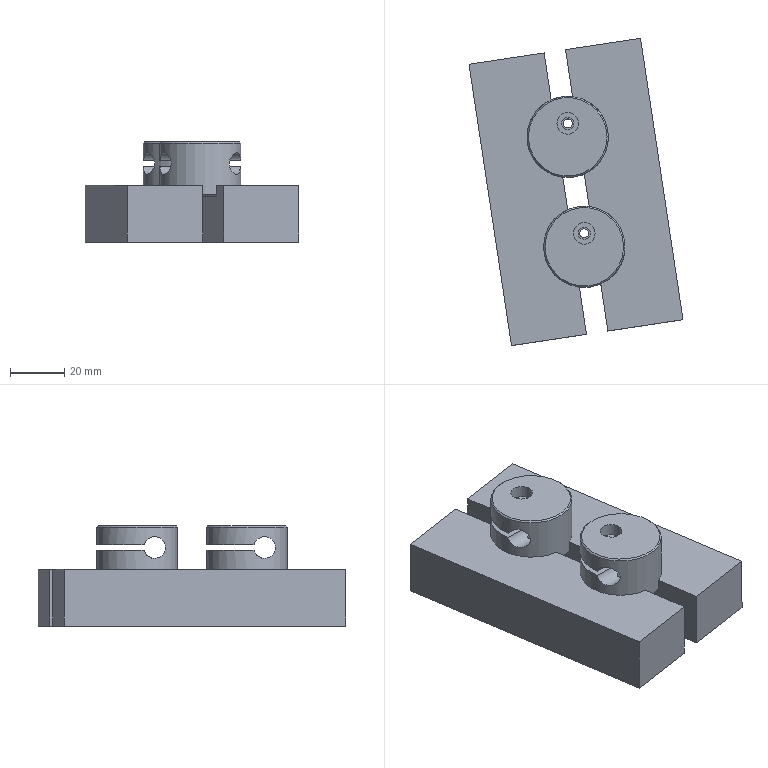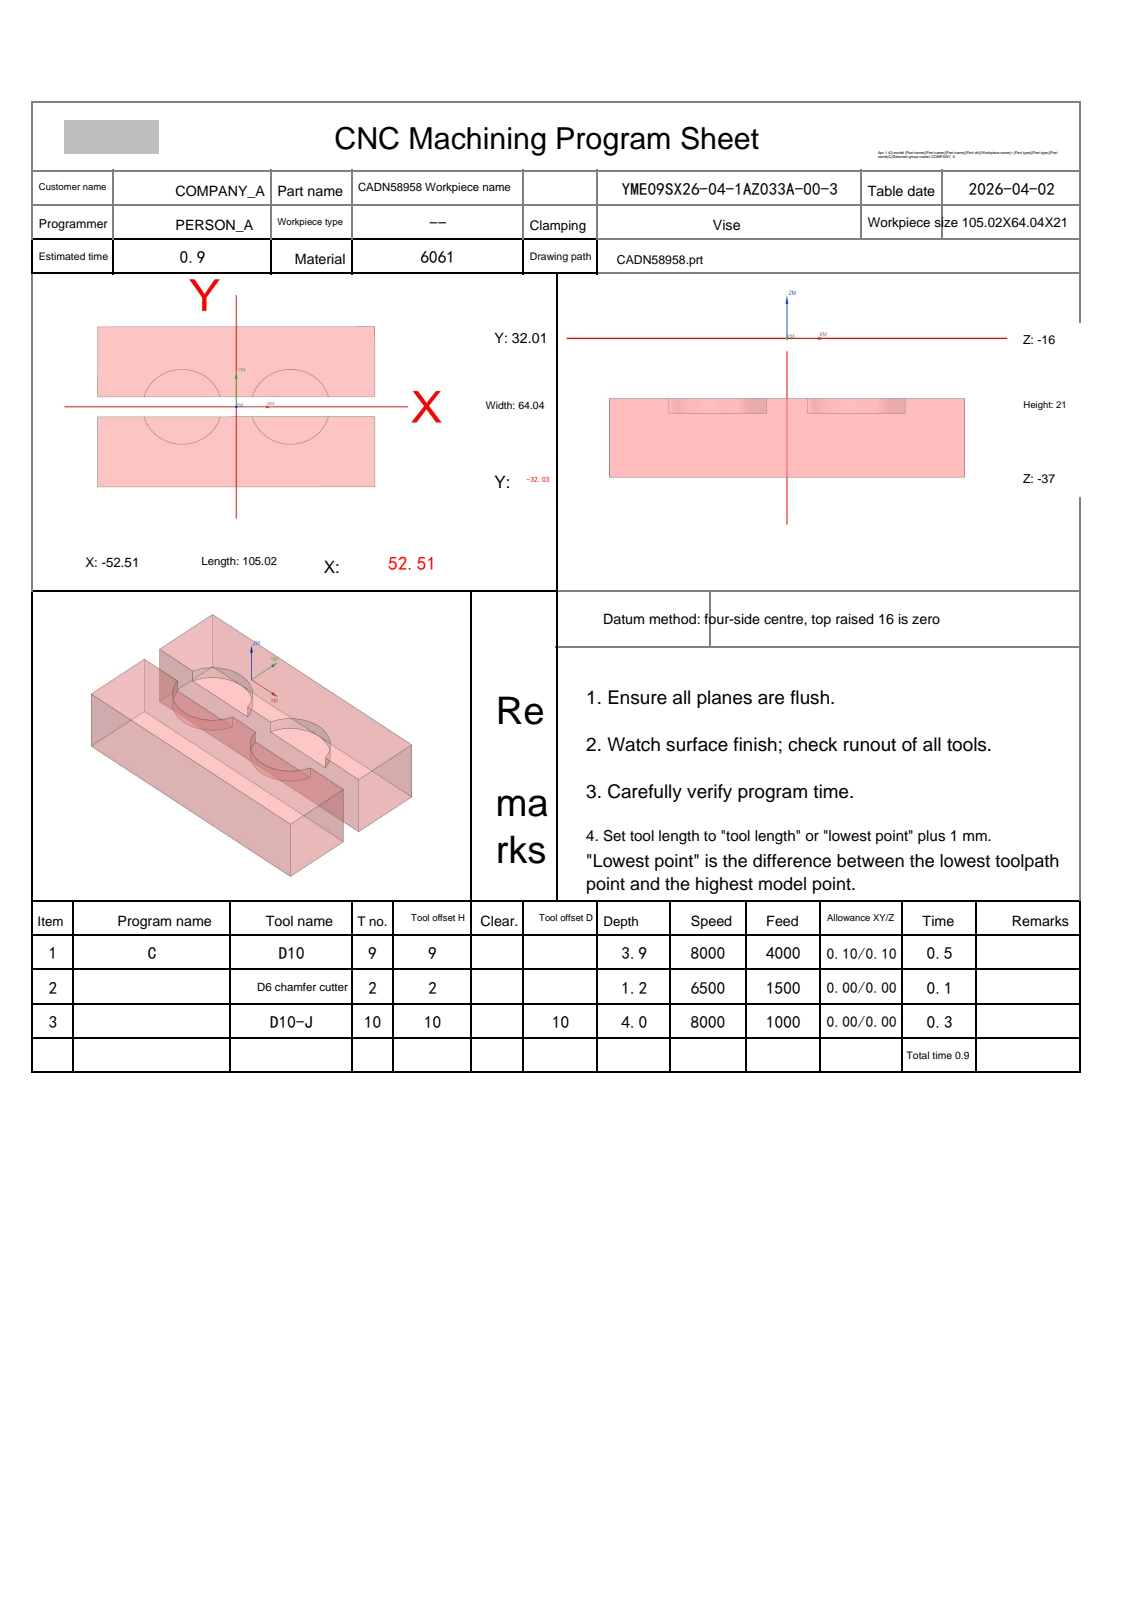NC program | NX | posted by the shop | part box 78.946 x 113.372 x 37 mm
Whole program:
%
O0001
(Machine time: 1.48 MIN)
(===Total Tool:3===)
(T9=D10     D=10.  R=0.   D-  H09 Z=-19.9 )
(T2=D6 chamfer cutter   D=6.   R=0.   D-  H02 Z=-17.2 )
(T10=D10-J  D=10.  R=0.   D10 H10 Z=-20.  )
G80 G90 G17 G49 G40
G91 G28 Z0
M01
N1 T09 M06
(D10  D=10. R=0. H=09 ce=0.10 di=0.10)
G00 G90 G54 X-14.353 Y.923 M03 S8000
G43 H09 Z-5.9
M08
Z-14.42
G03 X-14.353 Y.923 Z-15.902 I-4.172 J-1.686 F4000.
X-22.862 Y.435 Z-16.489 I-4.172 J-1.686
G01 X-22.914 Y.248
G03 X-22.95 Y-.017 I.964 J-.265
X-22.914 Y-.282 I1. J0.0
G01 X-22.81 Y-.657
G03 X-20.497 Y-2.416 I2.313 J.641
X-18.184 Y-.655 I0.0 J2.4
G01 X-18.08 Y-.28
G03 X-18.045 Y-.016 I-.964 J.265
X-18.08 Y.25 I-1. J0.0
G01 X-18.184 Y.625
G03 X-20.497 Y2.384 I-2.313 J-.641
X-21.129 Y2.299 I0.0 J-2.4
G02 X-21.392 Y2.264 I-.263 J.965
G01 X-21.509 Y2.271
X-29.01 Y3.16
X-29.128 Y3.167
G03 X-30.091 Y2.433 I0.0 J-1.
G01 X-30.769 Y-.02
X-30.038 Y-2.66
G03 X-20.497 Y-9.916 I9.541 J2.643
X-10.955 Y-2.653 I0.0 J9.9
G01 X-10.225 Y-.012
X-10.957 Y2.627
G03 X-20.497 Y9.884 I-9.541 J-2.643
X-30.04 Y2.62 I0.0 J-9.9
G01 X-30.769 Y-.02
X-30.113 Y-2.386
X-30.038 Y-2.66
G03 X-29.978 Y-2.867 I9.541 J2.643
G01 X-27.105 Y-2.003
Z-14.989
G00 X-14.353 Y.923
G03 X-14.353 Y.923 Z-16.471 I-4.172 J-1.686
X-22.862 Y.435 Z-17.057 I-4.172 J-1.686
G01 X-22.914 Y.248
G03 X-22.95 Y-.017 I.964 J-.265
X-22.914 Y-.282 I1. J0.0
G01 X-22.81 Y-.657
G03 X-20.497 Y-2.416 I2.313 J.641
X-18.184 Y-.655 I0.0 J2.4
G01 X-18.08 Y-.28
G03 X-18.045 Y-.016 I-.964 J.265
X-18.08 Y.25 I-1. J0.0
G01 X-18.184 Y.625
G03 X-20.497 Y2.384 I-2.313 J-.641
X-21.129 Y2.299 I0.0 J-2.4
G02 X-21.392 Y2.264 I-.263 J.965
G01 X-21.509 Y2.271
X-29.01 Y3.16
X-29.128 Y3.167
G03 X-30.091 Y2.433 I0.0 J-1.
G01 X-30.769 Y-.02
X-30.038 Y-2.66
G03 X-20.497 Y-9.916 I9.541 J2.643
X-10.955 Y-2.653 I0.0 J9.9
G01 X-10.225 Y-.012
X-10.957 Y2.627
G03 X-20.497 Y9.884 I-9.541 J-2.643
X-30.04 Y2.62 I0.0 J-9.9
G01 X-30.769 Y-.02
X-30.113 Y-2.386
X-30.038 Y-2.66
G03 X-29.978 Y-2.867 I9.541 J2.643
G01 X-27.105 Y-2.003
Z-15.557
G00 X-14.353 Y.923
G03 X-14.353 Y.923 Z-17.039 I-4.172 J-1.686
X-22.862 Y.435 Z-17.626 I-4.172 J-1.686
G01 X-22.914 Y.248
G03 X-22.95 Y-.017 I.964 J-.265
X-22.914 Y-.282 I1. J0.0
G01 X-22.81 Y-.657
G03 X-20.497 Y-2.416 I2.313 J.641
X-18.184 Y-.655 I0.0 J2.4
G01 X-18.08 Y-.28
G03 X-18.045 Y-.016 I-.964 J.265
X-18.08 Y.25 I-1. J0.0
G01 X-18.184 Y.625
G03 X-20.497 Y2.384 I-2.313 J-.641
X-21.129 Y2.299 I0.0 J-2.4
G02 X-21.392 Y2.264 I-.263 J.965
G01 X-21.509 Y2.271
X-29.01 Y3.16
X-29.128 Y3.167
G03 X-30.091 Y2.433 I0.0 J-1.
G01 X-30.769 Y-.02
X-30.038 Y-2.66
G03 X-20.497 Y-9.916 I9.541 J2.643
X-10.955 Y-2.653 I0.0 J9.9
G01 X-10.225 Y-.012
X-10.957 Y2.627
G03 X-20.497 Y9.884 I-9.541 J-2.643
X-30.04 Y2.62 I0.0 J-9.9
G01 X-30.769 Y-.02
X-30.113 Y-2.386
X-30.038 Y-2.66
G03 X-29.978 Y-2.867 I9.541 J2.643
G01 X-27.105 Y-2.003
Z-16.126
G00 X-14.353 Y.923
G03 X-14.353 Y.923 Z-17.608 I-4.172 J-1.686
X-22.862 Y.435 Z-18.194 I-4.172 J-1.686
G01 X-22.914 Y.248
G03 X-22.95 Y-.017 I.964 J-.265
X-22.914 Y-.282 I1. J0.0
G01 X-22.81 Y-.657
G03 X-20.497 Y-2.416 I2.313 J.641
X-18.184 Y-.655 I0.0 J2.4
G01 X-18.08 Y-.28
G03 X-18.045 Y-.016 I-.964 J.265
X-18.08 Y.25 I-1. J0.0
G01 X-18.184 Y.625
G03 X-20.497 Y2.384 I-2.313 J-.641
X-21.129 Y2.299 I0.0 J-2.4
G02 X-21.392 Y2.264 I-.263 J.965
G01 X-21.509 Y2.271
X-29.01 Y3.16
X-29.128 Y3.167
G03 X-30.091 Y2.433 I0.0 J-1.
G01 X-30.769 Y-.02
X-30.038 Y-2.66
G03 X-20.497 Y-9.916 I9.541 J2.643
X-10.955 Y-2.653 I0.0 J9.9
G01 X-10.225 Y-.012
X-10.957 Y2.627
G03 X-20.497 Y9.884 I-9.541 J-2.643
X-30.04 Y2.62 I0.0 J-9.9
G01 X-30.769 Y-.02
X-30.113 Y-2.386
X-30.038 Y-2.66
G03 X-29.978 Y-2.867 I9.541 J2.643
G01 X-27.105 Y-2.003
Z-16.694
G00 X-14.353 Y.923
G03 X-14.353 Y.923 Z-18.176 I-4.172 J-1.686
X-22.862 Y.435 Z-18.763 I-4.172 J-1.686
G01 X-22.914 Y.248
G03 X-22.95 Y-.017 I.964 J-.265
X-22.914 Y-.282 I1. J0.0
G01 X-22.81 Y-.657
G03 X-20.497 Y-2.416 I2.313 J.641
X-18.184 Y-.655 I0.0 J2.4
G01 X-18.08 Y-.28
G03 X-18.045 Y-.016 I-.964 J.265
X-18.08 Y.25 I-1. J0.0
G01 X-18.184 Y.625
G03 X-20.497 Y2.384 I-2.313 J-.641
X-21.129 Y2.299 I0.0 J-2.4
G02 X-21.392 Y2.264 I-.263 J.965
G01 X-21.509 Y2.271
X-29.01 Y3.16
X-29.128 Y3.167
G03 X-30.091 Y2.433 I0.0 J-1.
G01 X-30.769 Y-.02
X-30.038 Y-2.66
G03 X-20.497 Y-9.916 I9.541 J2.643
X-10.955 Y-2.653 I0.0 J9.9
G01 X-10.225 Y-.012
X-10.957 Y2.627
G03 X-20.497 Y9.884 I-9.541 J-2.643
X-30.04 Y2.62 I0.0 J-9.9
G01 X-30.769 Y-.02
X-30.113 Y-2.386
X-30.038 Y-2.66
G03 X-29.978 Y-2.867 I9.541 J2.643
G01 X-27.105 Y-2.003
Z-17.263
G00 X-14.353 Y.923
G03 X-14.353 Y.923 Z-18.745 I-4.172 J-1.686
X-22.862 Y.435 Z-19.331 I-4.172 J-1.686
G01 X-22.914 Y.248
G03 X-22.95 Y-.017 I.964 J-.265
X-22.914 Y-.282 I1. J0.0
G01 X-22.81 Y-.657
G03 X-20.497 Y-2.416 I2.313 J.641
X-18.184 Y-.655 I0.0 J2.4
G01 X-18.08 Y-.28
G03 X-18.045 Y-.016 I-.964 J.265
X-18.08 Y.25 I-1. J0.0
G01 X-18.184 Y.625
G03 X-20.497 Y2.384 I-2.313 J-.641
X-21.129 Y2.299 I0.0 J-2.4
G02 X-21.392 Y2.264 I-.263 J.965
G01 X-21.509 Y2.271
X-29.01 Y3.16
X-29.128 Y3.167
G03 X-30.091 Y2.433 I0.0 J-1.
G01 X-30.769 Y-.02
X-30.038 Y-2.66
G03 X-20.497 Y-9.916 I9.541 J2.643
X-10.955 Y-2.653 I0.0 J9.9
G01 X-10.225 Y-.012
X-10.957 Y2.627
G03 X-20.497 Y9.884 I-9.541 J-2.643
X-30.04 Y2.62 I0.0 J-9.9
G01 X-30.769 Y-.02
X-30.113 Y-2.386
X-30.038 Y-2.66
G03 X-29.978 Y-2.867 I9.541 J2.643
G01 X-27.105 Y-2.003
Z-17.831
G00 X-14.353 Y.923
G03 X-14.353 Y.923 Z-19.313 I-4.172 J-1.686
X-22.862 Y.435 Z-19.9 I-4.172 J-1.686
G01 X-22.914 Y.248
G03 X-22.95 Y-.017 I.964 J-.265
X-22.914 Y-.282 I1. J0.0
G01 X-22.81 Y-.657
G03 X-20.497 Y-2.416 I2.313 J.641
X-18.184 Y-.655 I0.0 J2.4
G01 X-18.08 Y-.28
G03 X-18.045 Y-.016 I-.964 J.265
X-18.08 Y.25 I-1. J0.0
G01 X-18.184 Y.625
G03 X-20.497 Y2.384 I-2.313 J-.641
X-21.129 Y2.299 I0.0 J-2.4
G02 X-21.392 Y2.264 I-.263 J.965
G01 X-21.509 Y2.271
X-29.01 Y3.16
X-29.128 Y3.167
G03 X-30.091 Y2.433 I0.0 J-1.
G01 X-30.769 Y-.02
X-30.038 Y-2.66
G03 X-20.497 Y-9.916 I9.541 J2.643
X-10.955 Y-2.653 I0.0 J9.9
G01 X-10.225 Y-.012
X-10.957 Y2.627
G03 X-20.497 Y9.884 I-9.541 J-2.643
X-30.04 Y2.62 I0.0 J-9.9
G01 X-30.769 Y-.02
X-30.113 Y-2.386
X-30.038 Y-2.66
G03 X-29.978 Y-2.867 I9.541 J2.643
G01 X-27.105 Y-2.003
Z-18.4
G00 Z-5.9
X14.358 Y-.941
Z-14.42
G03 X14.358 Y-.941 Z-15.902 I4.172 J1.686
X22.868 Y-.453 Z-16.489 I4.172 J1.686
G01 X22.92 Y-.265
G03 X22.955 Y-.001 I-.964 J.265
X22.92 Y.265 I-1. J0.0
G01 X22.816 Y.64
G03 X20.503 Y2.399 I-2.313 J-.641
X18.19 Y.638 I0.0 J-2.4
G01 X18.086 Y.263
G03 X18.05 Y-.002 I.964 J-.265
X18.086 Y-.267 I1. J0.0
G01 X18.19 Y-.642
G03 X20.503 Y-2.401 I2.313 J.641
X21.135 Y-2.316 I0.0 J2.4
G02 X21.398 Y-2.281 I.263 J-.965
G01 X21.515 Y-2.288
X29.016 Y-3.177
X29.133 Y-3.184
G03 X30.097 Y-2.45 I0.0 J1.
G01 X30.775 Y.003
X30.043 Y2.642
G03 X20.503 Y9.899 I-9.541 J-2.643
X10.96 Y2.635 I0.0 J-9.9
G01 X10.231 Y-.005
X10.962 Y-2.645
G03 X20.503 Y-9.901 I9.541 J2.643
X30.045 Y-2.638 I0.0 J9.9
G01 X30.775 Y.003
X30.119 Y2.369
X30.043 Y2.642
G03 X29.983 Y2.85 I-9.541 J-2.643
G01 X27.111 Y1.986
Z-14.989
G00 X15.819 Y-4.34
G03 X15.819 Y-4.34 Z-16.471 I2.712 J3.591
X22.868 Y.452 Z-17.057 I2.712 J3.591
G01 X22.816 Y.64
G03 X20.503 Y2.399 I-2.313 J-.641
X18.19 Y.638 I0.0 J-2.4
G01 X18.086 Y.263
G03 X18.05 Y-.002 I.964 J-.265
X18.086 Y-.267 I1. J0.0
G01 X18.19 Y-.642
G03 X20.503 Y-2.401 I2.313 J.641
X21.998 Y-1.879 I0.0 J2.4
G02 X22.239 Y-1.737 I.623 J-.783
G01 X29.513 Y1.263
G03 X30.132 Y2.188 I-.381 J.924
X30.095 Y2.455 I-1. J0.0
G01 X30.043 Y2.642
G03 X20.503 Y9.899 I-9.541 J-2.643
X10.96 Y2.635 I0.0 J-9.9
G01 X10.231 Y-.005
X10.962 Y-2.645
G03 X20.503 Y-9.901 I9.541 J2.643
X30.045 Y-2.638 I0.0 J9.9
G01 X30.775 Y.003
X30.043 Y2.642
G03 X27.708 Y6.788 I-9.541 J-2.643
X27.356 Y7.143 I-7.205 J-6.789
G01 X25.279 Y4.978
Z-15.557
G00 X15.819 Y-4.34
G03 X15.819 Y-4.34 Z-17.039 I2.712 J3.591
X22.868 Y.452 Z-17.626 I2.712 J3.591
G01 X22.816 Y.64
G03 X20.503 Y2.399 I-2.313 J-.641
X18.19 Y.638 I0.0 J-2.4
G01 X18.086 Y.263
G03 X18.05 Y-.002 I.964 J-.265
X18.086 Y-.267 I1. J0.0
G01 X18.19 Y-.642
G03 X20.503 Y-2.401 I2.313 J.641
X21.998 Y-1.879 I0.0 J2.4
G02 X22.239 Y-1.737 I.623 J-.783
G01 X29.513 Y1.263
G03 X30.132 Y2.188 I-.381 J.924
X30.095 Y2.455 I-1. J0.0
G01 X30.043 Y2.642
G03 X20.503 Y9.899 I-9.541 J-2.643
X10.96 Y2.635 I0.0 J-9.9
G01 X10.231 Y-.005
X10.962 Y-2.645
G03 X20.503 Y-9.901 I9.541 J2.643
X30.045 Y-2.638 I0.0 J9.9
G01 X30.775 Y.003
X30.043 Y2.642
G03 X27.708 Y6.788 I-9.541 J-2.643
X27.356 Y7.143 I-7.205 J-6.789
G01 X25.279 Y4.978
Z-16.126
G00 X15.819 Y-4.34
G03 X15.819 Y-4.34 Z-17.608 I2.712 J3.591
X22.868 Y.452 Z-18.194 I2.712 J3.591
G01 X22.816 Y.64
G03 X20.503 Y2.399 I-2.313 J-.641
X18.19 Y.638 I0.0 J-2.4
G01 X18.086 Y.263
G03 X18.05 Y-.002 I.964 J-.265
X18.086 Y-.267 I1. J0.0
G01 X18.19 Y-.642
G03 X20.503 Y-2.401 I2.313 J.641
X21.998 Y-1.879 I0.0 J2.4
G02 X22.239 Y-1.737 I.623 J-.783
G01 X29.513 Y1.263
G03 X30.132 Y2.188 I-.381 J.924
X30.095 Y2.455 I-1. J0.0
G01 X30.043 Y2.642
G03 X20.503 Y9.899 I-9.541 J-2.643
X10.96 Y2.635 I0.0 J-9.9
G01 X10.231 Y-.005
X10.962 Y-2.645
G03 X20.503 Y-9.901 I9.541 J2.643
X30.045 Y-2.638 I0.0 J9.9
G01 X30.775 Y.003
X30.043 Y2.642
G03 X27.708 Y6.788 I-9.541 J-2.643
X27.356 Y7.143 I-7.205 J-6.789
G01 X25.279 Y4.978
Z-16.694
G00 X15.819 Y-4.34
G03 X15.819 Y-4.34 Z-18.176 I2.712 J3.591
X22.868 Y.452 Z-18.763 I2.712 J3.591
G01 X22.816 Y.64
G03 X20.503 Y2.399 I-2.313 J-.641
X18.19 Y.638 I0.0 J-2.4
G01 X18.086 Y.263
G03 X18.05 Y-.002 I.964 J-.265
X18.086 Y-.267 I1. J0.0
G01 X18.19 Y-.642
G03 X20.503 Y-2.401 I2.313 J.641
X21.998 Y-1.879 I0.0 J2.4
G02 X22.239 Y-1.737 I.623 J-.783
G01 X29.513 Y1.263
G03 X30.132 Y2.188 I-.381 J.924
X30.095 Y2.455 I-1. J0.0
G01 X30.043 Y2.642
G03 X20.503 Y9.899 I-9.541 J-2.643
X10.96 Y2.635 I0.0 J-9.9
G01 X10.231 Y-.005
X10.962 Y-2.645
G03 X20.503 Y-9.901 I9.541 J2.643
X30.045 Y-2.638 I0.0 J9.9
G01 X30.775 Y.003
X30.043 Y2.642
G03 X27.708 Y6.788 I-9.541 J-2.643
X27.356 Y7.143 I-7.205 J-6.789
G01 X25.279 Y4.978
Z-17.263
G00 X15.819 Y-4.34
G03 X15.819 Y-4.34 Z-18.745 I2.712 J3.591
X22.868 Y.452 Z-19.331 I2.712 J3.591
G01 X22.816 Y.64
G03 X20.503 Y2.399 I-2.313 J-.641
X18.19 Y.638 I0.0 J-2.4
G01 X18.086 Y.263
G03 X18.05 Y-.002 I.964 J-.265
X18.086 Y-.267 I1. J0.0
G01 X18.19 Y-.642
G03 X20.503 Y-2.401 I2.313 J.641
X21.998 Y-1.879 I0.0 J2.4
G02 X22.239 Y-1.737 I.623 J-.783
G01 X29.513 Y1.263
G03 X30.132 Y2.188 I-.381 J.924
X30.095 Y2.455 I-1. J0.0
G01 X30.043 Y2.642
G03 X20.503 Y9.899 I-9.541 J-2.643
X10.96 Y2.635 I0.0 J-9.9
G01 X10.231 Y-.005
X10.962 Y-2.645
G03 X20.503 Y-9.901 I9.541 J2.643
X30.045 Y-2.638 I0.0 J9.9
G01 X30.775 Y.003
X30.043 Y2.642
G03 X27.708 Y6.788 I-9.541 J-2.643
X27.356 Y7.143 I-7.205 J-6.789
G01 X25.279 Y4.978
Z-17.831
G00 X15.819 Y-4.34
G03 X15.819 Y-4.34 Z-19.313 I2.712 J3.591
X22.868 Y.452 Z-19.9 I2.712 J3.591
G01 X22.816 Y.64
G03 X20.503 Y2.399 I-2.313 J-.641
X18.19 Y.638 I0.0 J-2.4
G01 X18.086 Y.263
G03 X18.05 Y-.002 I.964 J-.265
X18.086 Y-.267 I1. J0.0
G01 X18.19 Y-.642
G03 X20.503 Y-2.401 I2.313 J.641
X21.998 Y-1.879 I0.0 J2.4
G02 X22.239 Y-1.737 I.623 J-.783
G01 X29.513 Y1.263
G03 X30.132 Y2.188 I-.381 J.924
X30.095 Y2.455 I-1. J0.0
G01 X30.043 Y2.642
G03 X20.503 Y9.899 I-9.541 J-2.643
X10.96 Y2.635 I0.0 J-9.9
G01 X10.231 Y-.005
X10.962 Y-2.645
G03 X20.503 Y-9.901 I9.541 J2.643
X30.045 Y-2.638 I0.0 J9.9
G01 X30.775 Y.003
X30.043 Y2.642
G03 X27.708 Y6.788 I-9.541 J-2.643
X27.356 Y7.143 I-7.205 J-6.789
G01 X25.279 Y4.978
Z-18.4
G00 Z-5.9
G91 G28 Z0.0
M05
M09
G91 G28 Z0.0
M01
N2 T02 M06
(D6 chamfer cutter  D=6. R=0. H=02 ce=0.00 di=0.00)
G00 G90 G54 X-33.889 Y-3.318 M03 S6500
G43 H02 Z34.
M08
Z-15.876
G01 Z-17.2 F1500.
G03 X-33.994 Y-3.651 I1.849 J-.762
G01 X-34.008 Y-3.704
X-33.989 Y-3.754
G03 X-20.497 Y-14.016 I13.492 J3.738
X-7.003 Y-3.745 I0.0 J14.
G01 X-6.984 Y-3.694
X-6.998 Y-3.641
G03 X-7.102 Y-3.309 I-1.953 J-.43
G01 Z-15.876
G00 Z-6.
X5.7 Y-2.725
Z-15.883
G01 Z-17.2
G03 X5.952 Y-2.965 I1.499 J1.324
G01 X5.993 Y-3.001
X6.047 Y-3.006
G02 X7.011 Y-3.739 I0.0 J-1.
G03 X20.503 Y-14.001 I13.492 J3.738
X33.997 Y-3.73 I0.0 J14.
G01 X34.016 Y-3.679
X34.002 Y-3.626
G03 X33.898 Y-3.294 I-1.953 J-.43
G01 Z-15.876
G00 Z-6.
X-7.105 Y3.286
Z-15.876
G01 Z-17.2
G03 X-7.001 Y3.619 I-1.849 J.762
G01 X-6.986 Y3.671
X-7.005 Y3.722
G03 X-20.497 Y13.984 I-13.492 J-3.738
X-33.992 Y3.712 I0.0 J-14.
G01 X-34.011 Y3.661
X-33.996 Y3.609
G03 X-33.892 Y3.276 I1.953 J.43
G01 Z-15.876
G00 Z-6.
X33.895 Y3.301
Z-15.876
G01 Z-17.2
G03 X33.999 Y3.634 I-1.849 J.764
G01 X34.014 Y3.686
X33.995 Y3.737
G03 X20.503 Y13.999 I-13.492 J-3.738
X7.008 Y3.727 I0.0 J-14.
G01 X6.989 Y3.676
X7.004 Y3.624
G03 X7.109 Y3.291 I1.953 J.432
G01 Z-15.876
G00 Z34.
G91 G28 Z0.0
M05
M09
G91 G28 Z0.0
M01
N3 T10 M06
(D10-J  D=10. R=0. H=10 ce=5.00 di=0.00)
G00 G90 G54 X-18.24 Y.251 M03 S8000
G43 H10 Z34.
M08
Z-19.
G01 Z-20. F1000.
G41 D10
X-18.04
G03 X-16.041 Y2.251 I-.001 J2.
X-20.497 Y4.984 I-4.456 J-2.268
X-25.497 Y-.016 I0.0 J-5.
X-20.497 Y-5.016 I5. J0.0
X-16.039 Y-2.281 I0.0 J5.
G01 X-16.041 Y2.252
G03 X-16.29 Y2.685 I-4.456 J-2.268
X-17.973 Y3.605 I-1.683 J-1.081
X-19.053 Y3.288 I0.0 J-2.
G01 X-19.696 Y2.875
G40 X-19.864 Y2.767
Z-19.
G00 Z34.
X22.76 Y.266
Z-19.
G01 Z-20.
G41 D10
X22.96
G03 X24.959 Y2.266 I-.001 J2.
X20.503 Y4.999 I-4.456 J-2.268
X15.503 Y-.001 I0.0 J-5.
X20.503 Y-5.001 I5. J0.0
X24.961 Y-2.266 I0.0 J5.
G01 X24.959 Y2.267
G03 X24.71 Y2.7 I-4.456 J-2.268
X23.027 Y3.62 I-1.683 J-1.081
X21.947 Y3.303 I0.0 J-2.
G01 X21.304 Y2.89
G40 X21.136 Y2.782
Z-19.
G00 Z34.
G00 G90 X-13.241 Y1.237 M03 S8000
Z34.
Z-19.
G01 Z-20. F1000.
G41 D10
X-13.041
G03 X-11.041 Y3.237 I-.001 J2.
X-20.497 Y9.984 I-9.456 J-3.254
X-30.497 Y-.016 I0.0 J-10.
X-20.497 Y-10.016 I10. J0.0
X-11.039 Y-3.264 I0.0 J10.
G01 X-11.041 Y3.238
G03 X-11.216 Y3.707 I-9.456 J-3.254
X-13.072 Y4.962 I-1.856 J-.745
X-13.817 Y4.818 I0.0 J-2.
G01 X-14.053 Y4.724
G40 X-14.238 Y4.649
Z-19.
G00 Z34.
X27.759 Y1.252
Z-19.
G01 Z-20.
G41 D10
X27.959
G03 X29.959 Y3.252 I-.001 J2.
X20.503 Y9.999 I-9.456 J-3.254
X10.503 Y-.001 I0.0 J-10.
X20.503 Y-10.001 I10. J0.0
X29.961 Y-3.249 I0.0 J10.
G01 X29.959 Y3.253
G03 X29.784 Y3.722 I-9.456 J-3.254
X27.928 Y4.977 I-1.856 J-.745
X27.183 Y4.833 I0.0 J-2.
G01 X26.947 Y4.739
G40 X26.762 Y4.664
Z-19.
G00 Z34.
M05
M09
G91 G28 Z0.0
G91 G28 Y0.0
M30
%